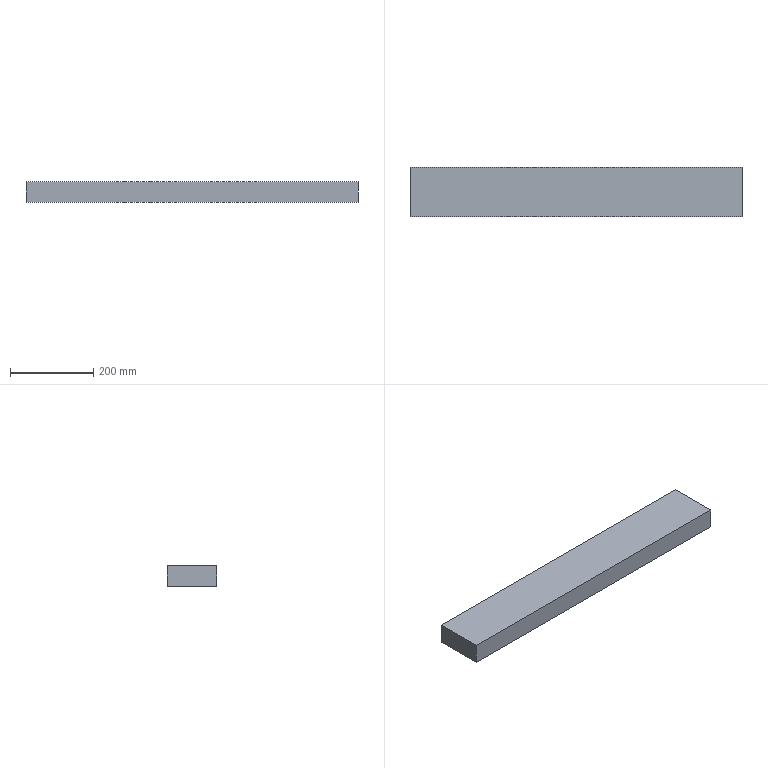Part | SolidWorks | features Extrusion 1 | 1 solid | 6 faces | box 800 x 120 x 50 mm | volume 4800000 mm3 | plane 6
STEP:
#1=CARTESIAN_POINT('',(-40.676,113.766,0.));
#2=VERTEX_POINT('',#1);
#3=CARTESIAN_POINT('',(-40.676,-6.234,0.));
#4=VERTEX_POINT('',#3);
#5=CARTESIAN_POINT('',(-40.676,113.766,0.));
#6=DIRECTION('',(0.,-1.,0.));
#7=VECTOR('',#6,1000.);
#8=LINE('',#5,#7);
#9=EDGE_CURVE('',#2,#4,#8,.T.);
#10=ORIENTED_EDGE('',*,*,#9,.T.);
#11=CARTESIAN_POINT('',(-40.676,-6.234,50.));
#12=VERTEX_POINT('',#11);
#13=CARTESIAN_POINT('',(-40.676,-6.234,50.));
#14=DIRECTION('',(0.,0.,-1.));
#15=VECTOR('',#14,1000.);
#16=LINE('',#13,#15);
#17=EDGE_CURVE('',#12,#4,#16,.T.);
#18=ORIENTED_EDGE('',*,*,#17,.F.);
#19=CARTESIAN_POINT('',(-40.676,113.766,50.));
#20=VERTEX_POINT('',#19);
#21=CARTESIAN_POINT('',(-40.676,113.766,50.));
#22=DIRECTION('',(0.,-1.,0.));
#23=VECTOR('',#22,1000.);
#24=LINE('',#21,#23);
#25=EDGE_CURVE('',#20,#12,#24,.T.);
#26=ORIENTED_EDGE('',*,*,#25,.F.);
#27=CARTESIAN_POINT('',(-40.676,113.766,50.));
#28=DIRECTION('',(0.,0.,-1.));
#29=VECTOR('',#28,1000.);
#30=LINE('',#27,#29);
#31=EDGE_CURVE('',#20,#2,#30,.T.);
#32=ORIENTED_EDGE('',*,*,#31,.T.);
#33=EDGE_LOOP('',(#10,#18,#26,#32));
#34=FACE_OUTER_BOUND('',#33,.T.);
#35=CARTESIAN_POINT('',(-40.676,113.766,50.));
#36=DIRECTION('',(1.,0.,0.));
#37=DIRECTION('',(0.,1.,0.));
#38=AXIS2_PLACEMENT_3D('',#35,#36,#37);
#39=PLANE('',#38);
#40=ADVANCED_FACE('',(#34),#39,.F.);
#41=CARTESIAN_POINT('',(759.324,-6.234,0.));
#42=VERTEX_POINT('',#41);
#43=CARTESIAN_POINT('',(-40.676,-6.234,0.));
#44=DIRECTION('',(1.,0.,0.));
#45=VECTOR('',#44,1000.);
#46=LINE('',#43,#45);
#47=EDGE_CURVE('',#4,#42,#46,.T.);
#48=ORIENTED_EDGE('',*,*,#47,.T.);
#49=CARTESIAN_POINT('',(759.324,-6.234,50.));
#50=VERTEX_POINT('',#49);
#51=CARTESIAN_POINT('',(759.324,-6.234,50.));
#52=DIRECTION('',(0.,0.,-1.));
#53=VECTOR('',#52,1000.);
#54=LINE('',#51,#53);
#55=EDGE_CURVE('',#50,#42,#54,.T.);
#56=ORIENTED_EDGE('',*,*,#55,.F.);
#57=CARTESIAN_POINT('',(-40.676,-6.234,50.));
#58=DIRECTION('',(1.,0.,0.));
#59=VECTOR('',#58,1000.);
#60=LINE('',#57,#59);
#61=EDGE_CURVE('',#12,#50,#60,.T.);
#62=ORIENTED_EDGE('',*,*,#61,.F.);
#63=ORIENTED_EDGE('',*,*,#17,.T.);
#64=EDGE_LOOP('',(#48,#56,#62,#63));
#65=FACE_OUTER_BOUND('',#64,.T.);
#66=CARTESIAN_POINT('',(-40.676,-6.234,50.));
#67=DIRECTION('',(0.,1.,0.));
#68=DIRECTION('',(0.,0.,1.));
#69=AXIS2_PLACEMENT_3D('',#66,#67,#68);
#70=PLANE('',#69);
#71=ADVANCED_FACE('',(#65),#70,.F.);
#72=CARTESIAN_POINT('',(759.324,113.766,0.));
#73=VERTEX_POINT('',#72);
#74=CARTESIAN_POINT('',(759.324,113.766,0.));
#75=DIRECTION('',(0.,1.,0.));
#76=VECTOR('',#75,1000.);
#77=LINE('',#74,#76);
#78=EDGE_CURVE('',#42,#73,#77,.T.);
#79=ORIENTED_EDGE('',*,*,#78,.T.);
#80=CARTESIAN_POINT('',(759.324,113.766,50.));
#81=VERTEX_POINT('',#80);
#82=CARTESIAN_POINT('',(759.324,113.766,50.));
#83=DIRECTION('',(0.,0.,-1.));
#84=VECTOR('',#83,1000.);
#85=LINE('',#82,#84);
#86=EDGE_CURVE('',#81,#73,#85,.T.);
#87=ORIENTED_EDGE('',*,*,#86,.F.);
#88=CARTESIAN_POINT('',(759.324,113.766,50.));
#89=DIRECTION('',(0.,1.,0.));
#90=VECTOR('',#89,1000.);
#91=LINE('',#88,#90);
#92=EDGE_CURVE('',#50,#81,#91,.T.);
#93=ORIENTED_EDGE('',*,*,#92,.F.);
#94=ORIENTED_EDGE('',*,*,#55,.T.);
#95=EDGE_LOOP('',(#79,#87,#93,#94));
#96=FACE_OUTER_BOUND('',#95,.T.);
#97=CARTESIAN_POINT('',(759.324,113.766,50.));
#98=DIRECTION('',(-1.,0.,0.));
#99=DIRECTION('',(0.,0.,1.));
#100=AXIS2_PLACEMENT_3D('',#97,#98,#99);
#101=PLANE('',#100);
#102=ADVANCED_FACE('',(#96),#101,.F.);
#103=CARTESIAN_POINT('',(-40.676,113.766,0.));
#104=DIRECTION('',(-1.,0.,0.));
#105=VECTOR('',#104,1000.);
#106=LINE('',#103,#105);
#107=EDGE_CURVE('',#73,#2,#106,.T.);
#108=ORIENTED_EDGE('',*,*,#107,.T.);
#109=ORIENTED_EDGE('',*,*,#31,.F.);
#110=CARTESIAN_POINT('',(-40.676,113.766,50.));
#111=DIRECTION('',(-1.,0.,0.));
#112=VECTOR('',#111,1000.);
#113=LINE('',#110,#112);
#114=EDGE_CURVE('',#81,#20,#113,.T.);
#115=ORIENTED_EDGE('',*,*,#114,.F.);
#116=ORIENTED_EDGE('',*,*,#86,.T.);
#117=EDGE_LOOP('',(#108,#109,#115,#116));
#118=FACE_OUTER_BOUND('',#117,.T.);
#119=CARTESIAN_POINT('',(-40.676,113.766,50.));
#120=DIRECTION('',(0.,-1.,0.));
#121=DIRECTION('',(0.,0.,-1.));
#122=AXIS2_PLACEMENT_3D('',#119,#120,#121);
#123=PLANE('',#122);
#124=ADVANCED_FACE('',(#118),#123,.F.);
#125=ORIENTED_EDGE('',*,*,#25,.T.);
#126=ORIENTED_EDGE('',*,*,#61,.T.);
#127=ORIENTED_EDGE('',*,*,#92,.T.);
#128=ORIENTED_EDGE('',*,*,#114,.T.);
#129=EDGE_LOOP('',(#125,#126,#127,#128));
#130=FACE_OUTER_BOUND('',#129,.T.);
#131=CARTESIAN_POINT('',(0.,0.,50.));
#132=DIRECTION('',(0.,0.,1.));
#133=DIRECTION('',(1.,0.,0.));
#134=AXIS2_PLACEMENT_3D('',#131,#132,#133);
#135=PLANE('',#134);
#136=ADVANCED_FACE('',(#130),#135,.T.);
#137=ORIENTED_EDGE('',*,*,#9,.F.);
#138=ORIENTED_EDGE('',*,*,#107,.F.);
#139=ORIENTED_EDGE('',*,*,#78,.F.);
#140=ORIENTED_EDGE('',*,*,#47,.F.);
#141=EDGE_LOOP('',(#137,#138,#139,#140));
#142=FACE_OUTER_BOUND('',#141,.T.);
#143=CARTESIAN_POINT('',(0.,0.,0.));
#144=DIRECTION('',(0.,0.,1.));
#145=DIRECTION('',(1.,0.,0.));
#146=AXIS2_PLACEMENT_3D('',#143,#144,#145);
#147=PLANE('',#146);
#148=ADVANCED_FACE('',(#142),#147,.F.);
#149=CLOSED_SHELL('',(#40,#71,#102,#124,#136,#148));
#150=MANIFOLD_SOLID_BREP('',#149);
#151=CARTESIAN_POINT('',(0.,0.,0.));
#152=DIRECTION('',(0.,0.,1.));
#153=DIRECTION('',(1.,0.,0.));
#154=AXIS2_PLACEMENT_3D('',#151,#152,#153);
#155=(LENGTH_UNIT()NAMED_UNIT(*)SI_UNIT(.MILLI.,.METRE.));
#156=UNCERTAINTY_MEASURE_WITH_UNIT(LENGTH_MEASURE(0.00001),#155,'','');
#157=(NAMED_UNIT(*)PLANE_ANGLE_UNIT()SI_UNIT($,.RADIAN.));
#158=(NAMED_UNIT(*)SI_UNIT($,.STERADIAN.)SOLID_ANGLE_UNIT());
#159=(GEOMETRIC_REPRESENTATION_CONTEXT(3)GLOBAL_UNCERTAINTY_ASSIGNED_CONTEXT((#156))GLOBAL_UNIT_ASSIGNED_CONTEXT((#155,#157,#158))REPRESENTATION_CONTEXT('',''));
#160=ADVANCED_BREP_SHAPE_REPRESENTATION('',(#150,#154),#159);